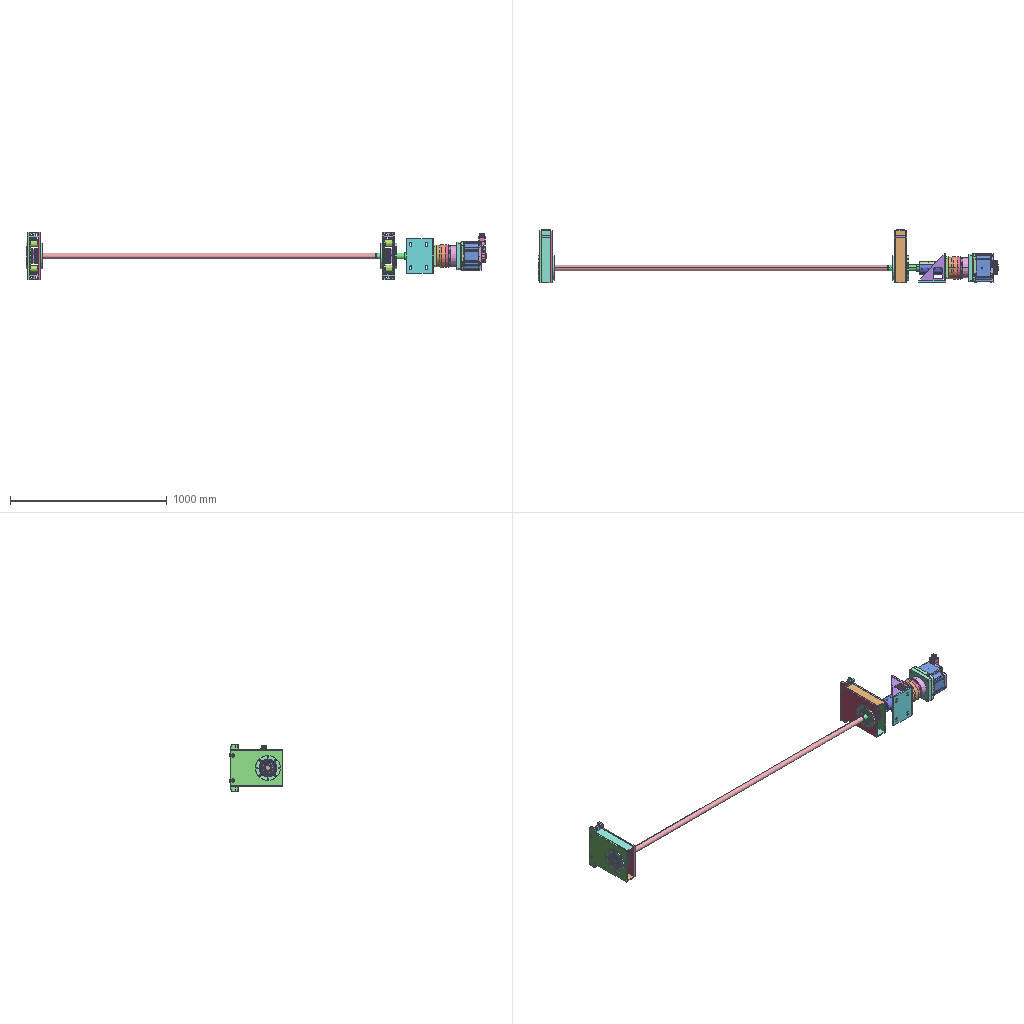Assembly | SolidWorks | 18 different items | 47 placed | box 2933 x 340 x 300 mm
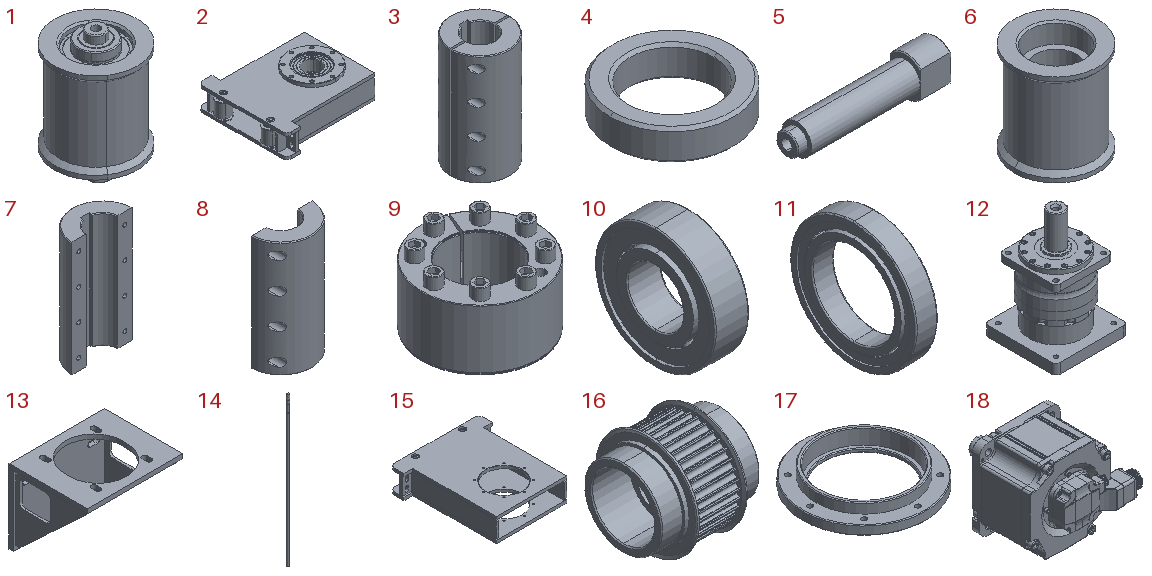Parts list (item | name | quantity | parent item | size | volume | features):
1 | (subassembly) | x4 | in 2 | 50 x 50 x 75 mm | 77764 mm3 | -
2 | (subassembly) | x2 | - | 340 x 300 x 104 mm | 2603051 mm3 | features LocalLPattern 1, ReferencePattern 1
3 | (subassembly) | x1 | - | 79.944 x 80 x 150 mm | 522394 mm3 | -
4 | - | x4 | in 1 | 22 x 22 x 5.5 mm | 1090 mm3 | features Chamfer 1, Extrusion 1
5 | - | x4 | in 1 | 75 x 15 x 20 mm | 13956 mm3 | features Chamfer 3, ICE 3, HoleWzd 1, Revolution 1
6 | - | x4 | in 1 | 50 x 50 x 55 mm | 55634 mm3 | features ICE 3, Chamfer 2, Extrusion 1, MirrorPattern 1
7 | - | x1 | in 3 | 79.944 x 38.5 x 150 mm | 263173 mm3 | features Chamfer 1, Extrusion 1, HoleWzd 1, ICE 1, LPattern 1
8 | - | x1 | in 3 | 79.944 x 38.5 x 150 mm | 259221 mm3 | features ICE 2, Chamfer 1, Extrusion 1, HoleWzd 1, LPattern 1
9 | - | x2 | - | 60 x 60 x 37 mm | 40890 mm3 | features CirPattern 2, Fillet 2, ICE 2, RevCut 2, Revolution 2, CutThin 1, Extrusion 1
10 | - | x8 | in 1 | 9 x 32 x 32 mm | 3542 mm3 | features BaseBody 1
11 | - | x4 | in 2 | 20 x 115 x 115 mm | 81153 mm3 | features Revolution 6, CirPattern 2, RevCut 2, MirrorPattern 1
12 | - | x1 | - | 175 x 175 x 271 mm | 3039277 mm3 | features MBimport 1
13 | - | x1 | - | 220 x 180 x 170 mm | 670263 mm3 | features ICE 8, CirPattern 1, Extrusion 1, LPattern 1, MirrorSolid 1, WeldmentFeature 1
14 | - | x1 | - | 40 x 40 x 2490 mm | 2423592 mm3 | features Chamfer 6, ICE 6, Extrusion 1, MoveFace 1
15 | - | x2 | in 2 | 300 x 330 x 80 mm | 1723505 mm3 | features ICE 11, Chamfer 4, CirPattern 2, HoleWzd 2, LPattern 2, Extrusion 1, Fillet 1, MirrorSolid 1, WeldmentFeature 1
16 | - | x2 | in 2 | 95 x 99 x 99 mm | 277778 mm3 | features ICE 8, Chamfer 4, Cut 2, Revolution 2, CirPattern 1, MirrorPattern 1, MirrorSolid 1, RefAxis 1
17 | - | x4 | in 2 | 160 x 160 x 25 mm | 141973 mm3 | features ICE 2, Chamfer 1, CirPattern 1, Extrusion 1, HoleWzd 1
18 | - | x1 | - | - | - | features MBimport 1
Mates (type | each side: item.copy, entity, surface, feature):
In the top assembly
Concentric | 14.1 face cylinder Boss-Extrude1 | 18.1 face cylinder
Concentric | 18.1 face cylinder | 12.1 face cylinder | 2 times
Coincident | 18.1 face plane | 12.1 face plane
Concentric | 14.1 face cylinder Boss-Extrude1 | 16.1 face cylinder Cut-Extrude7
Concentric | 14.1 face cylinder Boss-Extrude1 | 16.2 face cylinder Cut-Extrude5
Width | assembly face | assembly face | 12.1 face plane | 12.1 face plane
Concentric | 16.1 face cylinder Cut-Extrude5 | 9.1 face cylinder Revolve1
Coincident | 16.1 face plane Cut-Extrude5 | 9.1 face plane Revolve1
Coincident | 16.2 face plane Cut-Extrude5 | 9.2 face plane Revolve1
Concentric | 16.2 face cylinder Cut-Extrude5 | 9.2 face cylinder Revolve1
DistanceDim | 12.1 face plane | 14.1 face plane Boss-Extrude1
Parallel | 13.1 face plane Boss-Extrude1 | 12.1 face plane | 2 times
Coincident | 13.1 face plane Boss-Extrude1 | 12.1 face plane
Slot | 13.1 face cylinder Cut-Extrude4 | 12.1 face cylinder
Coincident | 13.1 face plane Boss-Extrude2 | assembly plane
Coincident | 14.1 face plane Boss-Extrude2 | 9.1 face plane Revolve1
Concentric | 12.1 face cylinder | 8.1 face cylinder Boss-Extrude1
Coincident | 12.1 face plane | 7.1 face plane Boss-Extrude1
Coincident | 15.1 face plane Boss-Extrude3 | assembly face
Width | 15.1 face plane Boss-Extrude3 | 15.1 face plane Boss-Extrude3 | 12.1 face plane | 12.1 face plane
DistanceDim | assembly face | 15.1 face plane Boss-Extrude3
In subassembly 2
Concentric | 16.3 face cylinder Cut-Extrude6 | 11.1 face cylinder Boss-Revolve4
Coincident | 16.3 face plane Cut-Extrude6 | 11.1 face plane Boss-Revolve4
Concentric | 17.1 face cylinder Boss-Extrude1 | 11.1 face cylinder Boss-Revolve3
Concentric | 16.3 face cylinder Boss-Extrude3 | 11.2 face cylinder Boss-Revolve4
Coincident | 16.3 face plane Boss-Extrude2 | 11.2 face plane Boss-Revolve4
Width | 15.2 face plane Boss-Extrude1 | 15.2 face plane Boss-Extrude3 | 16.3 face plane Boss-Extrude3 | 16.3 face plane Boss-Extrude1
Concentric | 15.2 face cylinder Cut-Extrude2 | 16.3 face cylinder Cut-Extrude5
Coincident | 15.2 face plane Boss-Extrude1 | 17.2 face plane Boss-Extrude2
Coincident | 15.2 face plane Boss-Extrude3 | 17.1 face plane Boss-Extrude2
Concentric | 15.2 face cylinder CirPattern2 | 17.1 face cylinder CirPattern1
Coincident | 15.2 face plane Boss-Extrude3 | 4.1 face plane Boss-Extrude1
Concentric | 15.2 face cylinder Cut-Extrude4 | 5.1 face cylinder Boss-Extrude2
Parallel | 5.1 face plane Cut-Extrude1 | 15.2 face plane Boss-Extrude6
In subassembly 1
Concentric | 5.2 face cylinder Revolve1 | 6.1 face cylinder Cut-Extrude1
Concentric | 5.2 face cylinder Revolve1 | 4.2 face cylinder Boss-Extrude1
Concentric | 5.2 face cylinder Revolve1 | 10.1 face cylinder Input1
Coincident | 5.2 face plane Boss-Extrude2 | 10.1 face plane Input1
Coincident | 6.1 face plane Cut-Extrude2 | 10.1 face plane Input1
Coincident | 6.1 face plane Mirror1 | 10.2 face plane Input1
Concentric | 5.2 face cylinder Revolve1 | 10.2 face cylinder Input1
Coincident | 4.2 face plane Boss-Extrude1 | 10.2 face plane Input1
In subassembly 3
Concentric | 7.2 face cylinder Boss-Extrude1 | 8.2 face cylinder Boss-Extrude1
Parallel | 7.2 face plane Cut-Extrude1 | 8.2 face plane Cut-Extrude1
Coincident | 7.2 face plane Boss-Extrude1 | 8.2 face plane Boss-Extrude1